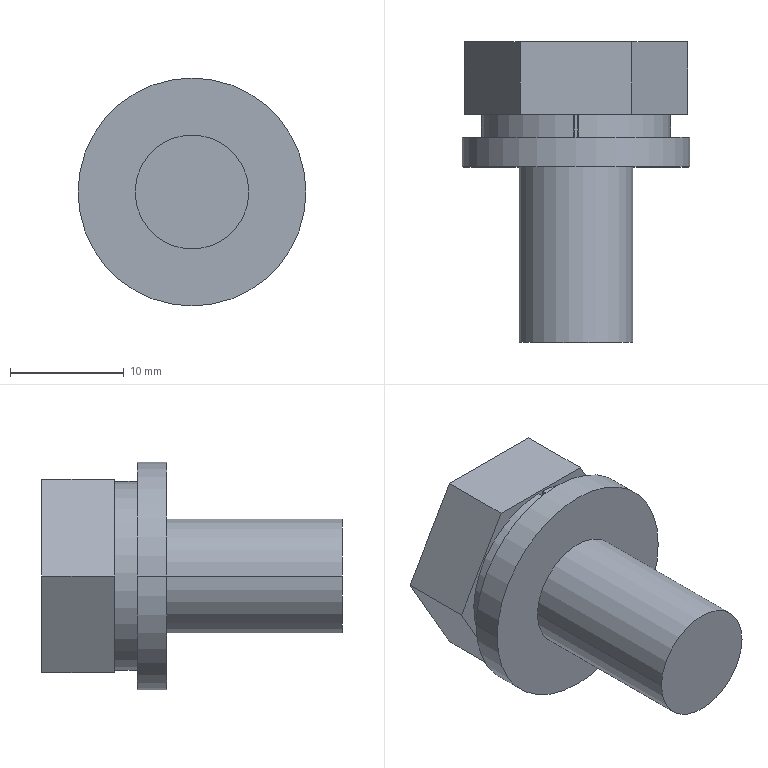Part | STEP file | LIB_68343151_M10X20 | 1 solid | 19 faces | box 20 x 26.4 x 20 mm | volume 4058 mm3 | plane 13 | cylinder 6 | commonest cylinder face diameters 10 x3 20 x2 16.6 x1
STEP:
#1=CARTESIAN_POINT('',(0.,0.,0.));
#2=DIRECTION('',(0.,0.,1.));
#3=DIRECTION('',(1.,0.,0.));
#4=AXIS2_PLACEMENT_3D('',#1,#2,#3);
#5=CARTESIAN_POINT('',(-4.907,0.,-8.5));
#6=VERTEX_POINT('',#5);
#7=CARTESIAN_POINT('',(-9.815,0.,0.));
#8=VERTEX_POINT('',#7);
#9=CARTESIAN_POINT('',(-4.907,0.,-8.5));
#10=DIRECTION('',(-0.5,0.,0.866));
#11=VECTOR('',#10,1.);
#12=LINE('',#9,#11);
#13=CARTESIAN_POINT('',(0.,0.,0.));
#14=DIRECTION('',(0.,1.,0.));
#15=DIRECTION('',(1.,0.,0.));
#16=AXIS2_PLACEMENT_3D('',#13,#14,#15);
#17=PLANE('',#16);
#18=CARTESIAN_POINT('',(-4.907,8.5));
#19=DIRECTION('',(-0.5,-0.866));
#20=VECTOR('',#19,1.);
#21=LINE('',#18,#20);
#22=(GEOMETRIC_REPRESENTATION_CONTEXT(2)PARAMETRIC_REPRESENTATION_CONTEXT()REPRESENTATION_CONTEXT('',''));
#23=DEFINITIONAL_REPRESENTATION('',(#21),#22);
#24=PCURVE('',#17,#23);
#25=CARTESIAN_POINT('',(-4.907,0.,-8.5));
#26=DIRECTION('',(-0.866,0.,-0.5));
#27=DIRECTION('',(-0.5,0.,0.866));
#28=AXIS2_PLACEMENT_3D('',#25,#26,#27);
#29=PLANE('',#28);
#30=CARTESIAN_POINT('',(0.,0.));
#31=DIRECTION('',(1.,0.));
#32=VECTOR('',#31,1.);
#33=LINE('',#30,#32);
#34=(GEOMETRIC_REPRESENTATION_CONTEXT(2)PARAMETRIC_REPRESENTATION_CONTEXT()REPRESENTATION_CONTEXT('',''));
#35=DEFINITIONAL_REPRESENTATION('',(#33),#34);
#36=PCURVE('',#29,#35);
#37=SURFACE_CURVE('',#12,(#24,#36),.PCURVE_S1.);
#38=EDGE_CURVE('',#6,#8,#37,.T.);
#39=ORIENTED_EDGE('',*,*,#38,.T.);
#40=CARTESIAN_POINT('',(-4.907,0.,8.5));
#41=VERTEX_POINT('',#40);
#42=CARTESIAN_POINT('',(-9.815,0.,0.));
#43=DIRECTION('',(0.5,0.,0.866));
#44=VECTOR('',#43,1.);
#45=LINE('',#42,#44);
#46=CARTESIAN_POINT('',(-9.815,0.));
#47=DIRECTION('',(0.5,-0.866));
#48=VECTOR('',#47,1.);
#49=LINE('',#46,#48);
#50=(GEOMETRIC_REPRESENTATION_CONTEXT(2)PARAMETRIC_REPRESENTATION_CONTEXT()REPRESENTATION_CONTEXT('',''));
#51=DEFINITIONAL_REPRESENTATION('',(#49),#50);
#52=PCURVE('',#17,#51);
#53=CARTESIAN_POINT('',(-9.815,0.,0.));
#54=DIRECTION('',(-0.866,0.,0.5));
#55=DIRECTION('',(0.5,0.,0.866));
#56=AXIS2_PLACEMENT_3D('',#53,#54,#55);
#57=PLANE('',#56);
#58=CARTESIAN_POINT('',(0.,0.));
#59=DIRECTION('',(1.,0.));
#60=VECTOR('',#59,1.);
#61=LINE('',#58,#60);
#62=(GEOMETRIC_REPRESENTATION_CONTEXT(2)PARAMETRIC_REPRESENTATION_CONTEXT()REPRESENTATION_CONTEXT('',''));
#63=DEFINITIONAL_REPRESENTATION('',(#61),#62);
#64=PCURVE('',#57,#63);
#65=SURFACE_CURVE('',#45,(#52,#64),.PCURVE_S1.);
#66=EDGE_CURVE('',#8,#41,#65,.T.);
#67=ORIENTED_EDGE('',*,*,#66,.T.);
#68=CARTESIAN_POINT('',(4.907,0.,8.5));
#69=VERTEX_POINT('',#68);
#70=CARTESIAN_POINT('',(-4.907,0.,8.5));
#71=DIRECTION('',(1.,0.,0.));
#72=VECTOR('',#71,1.);
#73=LINE('',#70,#72);
#74=CARTESIAN_POINT('',(-4.907,-8.5));
#75=DIRECTION('',(1.,0.));
#76=VECTOR('',#75,1.);
#77=LINE('',#74,#76);
#78=(GEOMETRIC_REPRESENTATION_CONTEXT(2)PARAMETRIC_REPRESENTATION_CONTEXT()REPRESENTATION_CONTEXT('',''));
#79=DEFINITIONAL_REPRESENTATION('',(#77),#78);
#80=PCURVE('',#17,#79);
#81=CARTESIAN_POINT('',(-4.907,0.,8.5));
#82=DIRECTION('',(0.,0.,1.));
#83=DIRECTION('',(1.,0.,0.));
#84=AXIS2_PLACEMENT_3D('',#81,#82,#83);
#85=PLANE('',#84);
#86=CARTESIAN_POINT('',(0.,0.));
#87=DIRECTION('',(1.,0.));
#88=VECTOR('',#87,1.);
#89=LINE('',#86,#88);
#90=(GEOMETRIC_REPRESENTATION_CONTEXT(2)PARAMETRIC_REPRESENTATION_CONTEXT()REPRESENTATION_CONTEXT('',''));
#91=DEFINITIONAL_REPRESENTATION('',(#89),#90);
#92=PCURVE('',#85,#91);
#93=SURFACE_CURVE('',#73,(#80,#92),.PCURVE_S1.);
#94=EDGE_CURVE('',#41,#69,#93,.T.);
#95=ORIENTED_EDGE('',*,*,#94,.T.);
#96=CARTESIAN_POINT('',(9.815,0.,0.));
#97=VERTEX_POINT('',#96);
#98=CARTESIAN_POINT('',(4.907,0.,8.5));
#99=DIRECTION('',(0.5,0.,-0.866));
#100=VECTOR('',#99,1.);
#101=LINE('',#98,#100);
#102=CARTESIAN_POINT('',(4.907,-8.5));
#103=DIRECTION('',(0.5,0.866));
#104=VECTOR('',#103,1.);
#105=LINE('',#102,#104);
#106=(GEOMETRIC_REPRESENTATION_CONTEXT(2)PARAMETRIC_REPRESENTATION_CONTEXT()REPRESENTATION_CONTEXT('',''));
#107=DEFINITIONAL_REPRESENTATION('',(#105),#106);
#108=PCURVE('',#17,#107);
#109=CARTESIAN_POINT('',(4.907,0.,8.5));
#110=DIRECTION('',(0.866,0.,0.5));
#111=DIRECTION('',(0.5,0.,-0.866));
#112=AXIS2_PLACEMENT_3D('',#109,#110,#111);
#113=PLANE('',#112);
#114=CARTESIAN_POINT('',(0.,0.));
#115=DIRECTION('',(1.,0.));
#116=VECTOR('',#115,1.);
#117=LINE('',#114,#116);
#118=(GEOMETRIC_REPRESENTATION_CONTEXT(2)PARAMETRIC_REPRESENTATION_CONTEXT()REPRESENTATION_CONTEXT('',''));
#119=DEFINITIONAL_REPRESENTATION('',(#117),#118);
#120=PCURVE('',#113,#119);
#121=SURFACE_CURVE('',#101,(#108,#120),.PCURVE_S1.);
#122=EDGE_CURVE('',#69,#97,#121,.T.);
#123=ORIENTED_EDGE('',*,*,#122,.T.);
#124=CARTESIAN_POINT('',(4.907,0.,-8.5));
#125=VERTEX_POINT('',#124);
#126=CARTESIAN_POINT('',(9.815,0.,0.));
#127=DIRECTION('',(-0.5,0.,-0.866));
#128=VECTOR('',#127,1.);
#129=LINE('',#126,#128);
#130=CARTESIAN_POINT('',(9.815,0.));
#131=DIRECTION('',(-0.5,0.866));
#132=VECTOR('',#131,1.);
#133=LINE('',#130,#132);
#134=(GEOMETRIC_REPRESENTATION_CONTEXT(2)PARAMETRIC_REPRESENTATION_CONTEXT()REPRESENTATION_CONTEXT('',''));
#135=DEFINITIONAL_REPRESENTATION('',(#133),#134);
#136=PCURVE('',#17,#135);
#137=CARTESIAN_POINT('',(9.815,0.,0.));
#138=DIRECTION('',(0.866,0.,-0.5));
#139=DIRECTION('',(-0.5,0.,-0.866));
#140=AXIS2_PLACEMENT_3D('',#137,#138,#139);
#141=PLANE('',#140);
#142=CARTESIAN_POINT('',(0.,0.));
#143=DIRECTION('',(1.,0.));
#144=VECTOR('',#143,1.);
#145=LINE('',#142,#144);
#146=(GEOMETRIC_REPRESENTATION_CONTEXT(2)PARAMETRIC_REPRESENTATION_CONTEXT()REPRESENTATION_CONTEXT('',''));
#147=DEFINITIONAL_REPRESENTATION('',(#145),#146);
#148=PCURVE('',#141,#147);
#149=SURFACE_CURVE('',#129,(#136,#148),.PCURVE_S1.);
#150=EDGE_CURVE('',#97,#125,#149,.T.);
#151=ORIENTED_EDGE('',*,*,#150,.T.);
#152=CARTESIAN_POINT('',(4.907,0.,-8.5));
#153=DIRECTION('',(-1.,0.,0.));
#154=VECTOR('',#153,1.);
#155=LINE('',#152,#154);
#156=CARTESIAN_POINT('',(4.907,8.5));
#157=DIRECTION('',(-1.,0.));
#158=VECTOR('',#157,1.);
#159=LINE('',#156,#158);
#160=(GEOMETRIC_REPRESENTATION_CONTEXT(2)PARAMETRIC_REPRESENTATION_CONTEXT()REPRESENTATION_CONTEXT('',''));
#161=DEFINITIONAL_REPRESENTATION('',(#159),#160);
#162=PCURVE('',#17,#161);
#163=CARTESIAN_POINT('',(4.907,0.,-8.5));
#164=DIRECTION('',(0.,0.,-1.));
#165=DIRECTION('',(-1.,0.,0.));
#166=AXIS2_PLACEMENT_3D('',#163,#164,#165);
#167=PLANE('',#166);
#168=CARTESIAN_POINT('',(0.,0.));
#169=DIRECTION('',(1.,0.));
#170=VECTOR('',#169,1.);
#171=LINE('',#168,#170);
#172=(GEOMETRIC_REPRESENTATION_CONTEXT(2)PARAMETRIC_REPRESENTATION_CONTEXT()REPRESENTATION_CONTEXT('',''));
#173=DEFINITIONAL_REPRESENTATION('',(#171),#172);
#174=PCURVE('',#167,#173);
#175=SURFACE_CURVE('',#155,(#162,#174),.PCURVE_S1.);
#176=EDGE_CURVE('',#125,#6,#175,.T.);
#177=ORIENTED_EDGE('',*,*,#176,.T.);
#178=EDGE_LOOP('',(#39,#67,#95,#123,#151,#177));
#179=FACE_BOUND('',#178,.F.);
#180=CARTESIAN_POINT('',(-0.25,0.,8.296));
#181=VERTEX_POINT('',#180);
#182=CARTESIAN_POINT('',(0.25,0.,8.296));
#183=VERTEX_POINT('',#182);
#184=CARTESIAN_POINT('',(0.,0.,0.));
#185=DIRECTION('',(0.,-1.,0.));
#186=DIRECTION('',(-0.03012,0.,0.9995));
#187=AXIS2_PLACEMENT_3D('',#184,#185,#186);
#188=CIRCLE('',#187,8.3);
#189=CARTESIAN_POINT('',(-0.25,-8.296));
#190=CARTESIAN_POINT('',(-14.619,-7.863));
#191=CARTESIAN_POINT('',(-7.06,4.365));
#192=CARTESIAN_POINT('',(0.5,16.592));
#193=CARTESIAN_POINT('',(7.31,3.932));
#194=CARTESIAN_POINT('',(14.119,-8.729));
#195=CARTESIAN_POINT('',(-0.25,-8.296));
#196=(BOUNDED_CURVE()B_SPLINE_CURVE(2,(#189,#190,#191,#192,#193,#194,#195),.UNSPECIFIED.,.T.,.F.)B_SPLINE_CURVE_WITH_KNOTS((1,2,2,2,2,1),(-2.094,0.,2.094,4.189,6.283,8.378),.UNSPECIFIED.)CURVE()GEOMETRIC_REPRESENTATION_ITEM()RATIONAL_B_SPLINE_CURVE((1.,0.5,1.,0.5,1.,0.5,1.))REPRESENTATION_ITEM(''));
#197=(GEOMETRIC_REPRESENTATION_CONTEXT(2)PARAMETRIC_REPRESENTATION_CONTEXT()REPRESENTATION_CONTEXT('',''));
#198=DEFINITIONAL_REPRESENTATION('',(#196),#197);
#199=PCURVE('',#17,#198);
#200=CARTESIAN_POINT('',(0.,0.,0.));
#201=DIRECTION('',(0.,-1.,0.));
#202=DIRECTION('',(0.,0.,-1.));
#203=AXIS2_PLACEMENT_3D('',#200,#201,#202);
#204=CYLINDRICAL_SURFACE('',#203,8.3);
#205=CARTESIAN_POINT('',(3.172,0.));
#206=DIRECTION('',(1.,0.));
#207=VECTOR('',#206,1.);
#208=LINE('',#205,#207);
#209=(GEOMETRIC_REPRESENTATION_CONTEXT(2)PARAMETRIC_REPRESENTATION_CONTEXT()REPRESENTATION_CONTEXT('',''));
#210=DEFINITIONAL_REPRESENTATION('',(#208),#209);
#211=PCURVE('',#204,#210);
#212=SURFACE_CURVE('',#188,(#199,#211),.PCURVE_S1.);
#213=EDGE_CURVE('',#181,#183,#212,.T.);
#214=ORIENTED_EDGE('',*,*,#213,.T.);
#215=CARTESIAN_POINT('',(0.1506,0.,4.998));
#216=VERTEX_POINT('',#215);
#217=CARTESIAN_POINT('',(0.25,0.,8.296));
#218=DIRECTION('',(-0.03012,0.,-0.9995));
#219=VECTOR('',#218,1.);
#220=LINE('',#217,#219);
#221=CARTESIAN_POINT('',(0.25,-8.296));
#222=DIRECTION('',(-0.03012,0.9995));
#223=VECTOR('',#222,1.);
#224=LINE('',#221,#223);
#225=(GEOMETRIC_REPRESENTATION_CONTEXT(2)PARAMETRIC_REPRESENTATION_CONTEXT()REPRESENTATION_CONTEXT('',''));
#226=DEFINITIONAL_REPRESENTATION('',(#224),#225);
#227=PCURVE('',#17,#226);
#228=CARTESIAN_POINT('',(0.25,0.,8.296));
#229=DIRECTION('',(-0.9995,0.,0.03012));
#230=DIRECTION('',(-0.03012,0.,-0.9995));
#231=AXIS2_PLACEMENT_3D('',#228,#229,#230);
#232=PLANE('',#231);
#233=CARTESIAN_POINT('',(0.,0.));
#234=DIRECTION('',(1.,0.));
#235=VECTOR('',#234,1.);
#236=LINE('',#233,#235);
#237=(GEOMETRIC_REPRESENTATION_CONTEXT(2)PARAMETRIC_REPRESENTATION_CONTEXT()REPRESENTATION_CONTEXT('',''));
#238=DEFINITIONAL_REPRESENTATION('',(#236),#237);
#239=PCURVE('',#232,#238);
#240=SURFACE_CURVE('',#220,(#227,#239),.PCURVE_S1.);
#241=EDGE_CURVE('',#183,#216,#240,.T.);
#242=ORIENTED_EDGE('',*,*,#241,.T.);
#243=CARTESIAN_POINT('',(-0.1506,0.,4.998));
#244=VERTEX_POINT('',#243);
#245=CARTESIAN_POINT('',(0.,0.,0.));
#246=DIRECTION('',(0.,-1.,0.));
#247=DIRECTION('',(0.03012,0.,0.9995));
#248=AXIS2_PLACEMENT_3D('',#245,#246,#247);
#249=CIRCLE('',#248,5.);
#250=CARTESIAN_POINT('',(0.1506,-4.998));
#251=CARTESIAN_POINT('',(-8.506,-5.259));
#252=CARTESIAN_POINT('',(-4.403,2.368));
#253=CARTESIAN_POINT('',(-0.3012,9.995));
#254=CARTESIAN_POINT('',(4.253,2.629));
#255=CARTESIAN_POINT('',(8.807,-4.737));
#256=CARTESIAN_POINT('',(0.1506,-4.998));
#257=(BOUNDED_CURVE()B_SPLINE_CURVE(2,(#250,#251,#252,#253,#254,#255,#256),.UNSPECIFIED.,.T.,.F.)B_SPLINE_CURVE_WITH_KNOTS((1,2,2,2,2,1),(-2.094,0.,2.094,4.189,6.283,8.378),.UNSPECIFIED.)CURVE()GEOMETRIC_REPRESENTATION_ITEM()RATIONAL_B_SPLINE_CURVE((1.,0.5,1.,0.5,1.,0.5,1.))REPRESENTATION_ITEM(''));
#258=(GEOMETRIC_REPRESENTATION_CONTEXT(2)PARAMETRIC_REPRESENTATION_CONTEXT()REPRESENTATION_CONTEXT('',''));
#259=DEFINITIONAL_REPRESENTATION('',(#257),#258);
#260=PCURVE('',#17,#259);
#261=CARTESIAN_POINT('',(0.,0.,0.));
#262=DIRECTION('',(0.,-1.,0.));
#263=DIRECTION('',(1.,0.,0.));
#264=AXIS2_PLACEMENT_3D('',#261,#262,#263);
#265=CYLINDRICAL_SURFACE('',#264,5.);
#266=CARTESIAN_POINT('',(1.541,0.));
#267=DIRECTION('',(1.,0.));
#268=VECTOR('',#267,1.);
#269=LINE('',#266,#268);
#270=(GEOMETRIC_REPRESENTATION_CONTEXT(2)PARAMETRIC_REPRESENTATION_CONTEXT()REPRESENTATION_CONTEXT('',''));
#271=DEFINITIONAL_REPRESENTATION('',(#269),#270);
#272=PCURVE('',#265,#271);
#273=SURFACE_CURVE('',#249,(#260,#272),.PCURVE_S1.);
#274=EDGE_CURVE('',#216,#244,#273,.T.);
#275=ORIENTED_EDGE('',*,*,#274,.T.);
#276=CARTESIAN_POINT('',(-0.1506,0.,4.998));
#277=DIRECTION('',(-0.03012,0.,0.9995));
#278=VECTOR('',#277,1.);
#279=LINE('',#276,#278);
#280=CARTESIAN_POINT('',(-0.1506,-4.998));
#281=DIRECTION('',(-0.03012,-0.9995));
#282=VECTOR('',#281,1.);
#283=LINE('',#280,#282);
#284=(GEOMETRIC_REPRESENTATION_CONTEXT(2)PARAMETRIC_REPRESENTATION_CONTEXT()REPRESENTATION_CONTEXT('',''));
#285=DEFINITIONAL_REPRESENTATION('',(#283),#284);
#286=PCURVE('',#17,#285);
#287=CARTESIAN_POINT('',(-0.1506,0.,4.998));
#288=DIRECTION('',(0.9995,0.,0.03012));
#289=DIRECTION('',(-0.03012,0.,0.9995));
#290=AXIS2_PLACEMENT_3D('',#287,#288,#289);
#291=PLANE('',#290);
#292=CARTESIAN_POINT('',(0.,0.));
#293=DIRECTION('',(1.,0.));
#294=VECTOR('',#293,1.);
#295=LINE('',#292,#294);
#296=(GEOMETRIC_REPRESENTATION_CONTEXT(2)PARAMETRIC_REPRESENTATION_CONTEXT()REPRESENTATION_CONTEXT('',''));
#297=DEFINITIONAL_REPRESENTATION('',(#295),#296);
#298=PCURVE('',#291,#297);
#299=SURFACE_CURVE('',#279,(#286,#298),.PCURVE_S1.);
#300=EDGE_CURVE('',#244,#181,#299,.T.);
#301=ORIENTED_EDGE('',*,*,#300,.T.);
#302=EDGE_LOOP('',(#214,#242,#275,#301));
#303=FACE_BOUND('',#302,.F.);
#304=ADVANCED_FACE('',(#179,#303),#17,.F.);
#305=ORIENTED_EDGE('',*,*,#38,.F.);
#306=CARTESIAN_POINT('',(-4.907,6.4,-8.5));
#307=VERTEX_POINT('',#306);
#308=CARTESIAN_POINT('',(-4.907,0.,-8.5));
#309=DIRECTION('',(0.,1.,0.));
#310=VECTOR('',#309,1.);
#311=LINE('',#308,#310);
#312=CARTESIAN_POINT('',(0.,0.));
#313=DIRECTION('',(0.,1.));
#314=VECTOR('',#313,1.);
#315=LINE('',#312,#314);
#316=(GEOMETRIC_REPRESENTATION_CONTEXT(2)PARAMETRIC_REPRESENTATION_CONTEXT()REPRESENTATION_CONTEXT('',''));
#317=DEFINITIONAL_REPRESENTATION('',(#315),#316);
#318=PCURVE('',#29,#317);
#319=CARTESIAN_POINT('',(9.815,0.));
#320=DIRECTION('',(0.,1.));
#321=VECTOR('',#320,1.);
#322=LINE('',#319,#321);
#323=(GEOMETRIC_REPRESENTATION_CONTEXT(2)PARAMETRIC_REPRESENTATION_CONTEXT()REPRESENTATION_CONTEXT('',''));
#324=DEFINITIONAL_REPRESENTATION('',(#322),#323);
#325=PCURVE('',#167,#324);
#326=SURFACE_CURVE('',#311,(#318,#325),.PCURVE_S1.);
#327=EDGE_CURVE('',#6,#307,#326,.T.);
#328=ORIENTED_EDGE('',*,*,#327,.T.);
#329=CARTESIAN_POINT('',(-9.815,6.4,0.));
#330=VERTEX_POINT('',#329);
#331=CARTESIAN_POINT('',(-4.907,6.4,-8.5));
#332=DIRECTION('',(-0.5,0.,0.866));
#333=VECTOR('',#332,1.);
#334=LINE('',#331,#333);
#335=CARTESIAN_POINT('',(0.,6.4));
#336=DIRECTION('',(1.,0.));
#337=VECTOR('',#336,1.);
#338=LINE('',#335,#337);
#339=(GEOMETRIC_REPRESENTATION_CONTEXT(2)PARAMETRIC_REPRESENTATION_CONTEXT()REPRESENTATION_CONTEXT('',''));
#340=DEFINITIONAL_REPRESENTATION('',(#338),#339);
#341=PCURVE('',#29,#340);
#342=CARTESIAN_POINT('',(0.,6.4,0.));
#343=DIRECTION('',(0.,1.,0.));
#344=DIRECTION('',(1.,0.,0.));
#345=AXIS2_PLACEMENT_3D('',#342,#343,#344);
#346=PLANE('',#345);
#347=CARTESIAN_POINT('',(-4.907,8.5));
#348=DIRECTION('',(-0.5,-0.866));
#349=VECTOR('',#348,1.);
#350=LINE('',#347,#349);
#351=(GEOMETRIC_REPRESENTATION_CONTEXT(2)PARAMETRIC_REPRESENTATION_CONTEXT()REPRESENTATION_CONTEXT('',''));
#352=DEFINITIONAL_REPRESENTATION('',(#350),#351);
#353=PCURVE('',#346,#352);
#354=SURFACE_CURVE('',#334,(#341,#353),.PCURVE_S1.);
#355=EDGE_CURVE('',#307,#330,#354,.T.);
#356=ORIENTED_EDGE('',*,*,#355,.T.);
#357=CARTESIAN_POINT('',(-9.815,0.,0.));
#358=DIRECTION('',(0.,1.,0.));
#359=VECTOR('',#358,1.);
#360=LINE('',#357,#359);
#361=CARTESIAN_POINT('',(9.815,0.));
#362=DIRECTION('',(0.,1.));
#363=VECTOR('',#362,1.);
#364=LINE('',#361,#363);
#365=(GEOMETRIC_REPRESENTATION_CONTEXT(2)PARAMETRIC_REPRESENTATION_CONTEXT()REPRESENTATION_CONTEXT('',''));
#366=DEFINITIONAL_REPRESENTATION('',(#364),#365);
#367=PCURVE('',#29,#366);
#368=CARTESIAN_POINT('',(0.,0.));
#369=DIRECTION('',(0.,1.));
#370=VECTOR('',#369,1.);
#371=LINE('',#368,#370);
#372=(GEOMETRIC_REPRESENTATION_CONTEXT(2)PARAMETRIC_REPRESENTATION_CONTEXT()REPRESENTATION_CONTEXT('',''));
#373=DEFINITIONAL_REPRESENTATION('',(#371),#372);
#374=PCURVE('',#57,#373);
#375=SURFACE_CURVE('',#360,(#367,#374),.PCURVE_S1.);
#376=EDGE_CURVE('',#8,#330,#375,.T.);
#377=ORIENTED_EDGE('',*,*,#376,.F.);
#378=EDGE_LOOP('',(#305,#328,#356,#377));
#379=FACE_BOUND('',#378,.F.);
#380=ADVANCED_FACE('',(#379),#29,.T.);
#381=ORIENTED_EDGE('',*,*,#176,.F.);
#382=CARTESIAN_POINT('',(4.907,6.4,-8.5));
#383=VERTEX_POINT('',#382);
#384=CARTESIAN_POINT('',(4.907,0.,-8.5));
#385=DIRECTION('',(0.,1.,0.));
#386=VECTOR('',#385,1.);
#387=LINE('',#384,#386);
#388=CARTESIAN_POINT('',(0.,0.));
#389=DIRECTION('',(0.,1.));
#390=VECTOR('',#389,1.);
#391=LINE('',#388,#390);
#392=(GEOMETRIC_REPRESENTATION_CONTEXT(2)PARAMETRIC_REPRESENTATION_CONTEXT()REPRESENTATION_CONTEXT('',''));
#393=DEFINITIONAL_REPRESENTATION('',(#391),#392);
#394=PCURVE('',#167,#393);
#395=CARTESIAN_POINT('',(9.815,0.));
#396=DIRECTION('',(0.,1.));
#397=VECTOR('',#396,1.);
#398=LINE('',#395,#397);
#399=(GEOMETRIC_REPRESENTATION_CONTEXT(2)PARAMETRIC_REPRESENTATION_CONTEXT()REPRESENTATION_CONTEXT('',''));
#400=DEFINITIONAL_REPRESENTATION('',(#398),#399);
#401=PCURVE('',#141,#400);
#402=SURFACE_CURVE('',#387,(#394,#401),.PCURVE_S1.);
#403=EDGE_CURVE('',#125,#383,#402,.T.);
#404=ORIENTED_EDGE('',*,*,#403,.T.);
#405=CARTESIAN_POINT('',(4.907,6.4,-8.5));
#406=DIRECTION('',(-1.,0.,0.));
#407=VECTOR('',#406,1.);
#408=LINE('',#405,#407);
#409=CARTESIAN_POINT('',(0.,6.4));
#410=DIRECTION('',(1.,0.));
#411=VECTOR('',#410,1.);
#412=LINE('',#409,#411);
#413=(GEOMETRIC_REPRESENTATION_CONTEXT(2)PARAMETRIC_REPRESENTATION_CONTEXT()REPRESENTATION_CONTEXT('',''));
#414=DEFINITIONAL_REPRESENTATION('',(#412),#413);
#415=PCURVE('',#167,#414);
#416=CARTESIAN_POINT('',(4.907,8.5));
#417=DIRECTION('',(-1.,0.));
#418=VECTOR('',#417,1.);
#419=LINE('',#416,#418);
#420=(GEOMETRIC_REPRESENTATION_CONTEXT(2)PARAMETRIC_REPRESENTATION_CONTEXT()REPRESENTATION_CONTEXT('',''));
#421=DEFINITIONAL_REPRESENTATION('',(#419),#420);
#422=PCURVE('',#346,#421);
#423=SURFACE_CURVE('',#408,(#415,#422),.PCURVE_S1.);
#424=EDGE_CURVE('',#383,#307,#423,.T.);
#425=ORIENTED_EDGE('',*,*,#424,.T.);
#426=ORIENTED_EDGE('',*,*,#327,.F.);
#427=EDGE_LOOP('',(#381,#404,#425,#426));
#428=FACE_BOUND('',#427,.F.);
#429=ADVANCED_FACE('',(#428),#167,.T.);
#430=ORIENTED_EDGE('',*,*,#150,.F.);
#431=CARTESIAN_POINT('',(9.815,6.4,0.));
#432=VERTEX_POINT('',#431);
#433=CARTESIAN_POINT('',(9.815,0.,0.));
#434=DIRECTION('',(0.,1.,0.));
#435=VECTOR('',#434,1.);
#436=LINE('',#433,#435);
#437=CARTESIAN_POINT('',(0.,0.));
#438=DIRECTION('',(0.,1.));
#439=VECTOR('',#438,1.);
#440=LINE('',#437,#439);
#441=(GEOMETRIC_REPRESENTATION_CONTEXT(2)PARAMETRIC_REPRESENTATION_CONTEXT()REPRESENTATION_CONTEXT('',''));
#442=DEFINITIONAL_REPRESENTATION('',(#440),#441);
#443=PCURVE('',#141,#442);
#444=CARTESIAN_POINT('',(9.815,0.));
#445=DIRECTION('',(0.,1.));
#446=VECTOR('',#445,1.);
#447=LINE('',#444,#446);
#448=(GEOMETRIC_REPRESENTATION_CONTEXT(2)PARAMETRIC_REPRESENTATION_CONTEXT()REPRESENTATION_CONTEXT('',''));
#449=DEFINITIONAL_REPRESENTATION('',(#447),#448);
#450=PCURVE('',#113,#449);
#451=SURFACE_CURVE('',#436,(#443,#450),.PCURVE_S1.);
#452=EDGE_CURVE('',#97,#432,#451,.T.);
#453=ORIENTED_EDGE('',*,*,#452,.T.);
#454=CARTESIAN_POINT('',(9.815,6.4,0.));
#455=DIRECTION('',(-0.5,0.,-0.866));
#456=VECTOR('',#455,1.);
#457=LINE('',#454,#456);
#458=CARTESIAN_POINT('',(0.,6.4));
#459=DIRECTION('',(1.,0.));
#460=VECTOR('',#459,1.);
#461=LINE('',#458,#460);
#462=(GEOMETRIC_REPRESENTATION_CONTEXT(2)PARAMETRIC_REPRESENTATION_CONTEXT()REPRESENTATION_CONTEXT('',''));
#463=DEFINITIONAL_REPRESENTATION('',(#461),#462);
#464=PCURVE('',#141,#463);
#465=CARTESIAN_POINT('',(9.815,0.));
#466=DIRECTION('',(-0.5,0.866));
#467=VECTOR('',#466,1.);
#468=LINE('',#465,#467);
#469=(GEOMETRIC_REPRESENTATION_CONTEXT(2)PARAMETRIC_REPRESENTATION_CONTEXT()REPRESENTATION_CONTEXT('',''));
#470=DEFINITIONAL_REPRESENTATION('',(#468),#469);
#471=PCURVE('',#346,#470);
#472=SURFACE_CURVE('',#457,(#464,#471),.PCURVE_S1.);
#473=EDGE_CURVE('',#432,#383,#472,.T.);
#474=ORIENTED_EDGE('',*,*,#473,.T.);
#475=ORIENTED_EDGE('',*,*,#403,.F.);
#476=EDGE_LOOP('',(#430,#453,#474,#475));
#477=FACE_BOUND('',#476,.F.);
#478=ADVANCED_FACE('',(#477),#141,.T.);
#479=ORIENTED_EDGE('',*,*,#122,.F.);
#480=CARTESIAN_POINT('',(4.907,6.4,8.5));
#481=VERTEX_POINT('',#480);
#482=CARTESIAN_POINT('',(4.907,0.,8.5));
#483=DIRECTION('',(0.,1.,0.));
#484=VECTOR('',#483,1.);
#485=LINE('',#482,#484);
#486=CARTESIAN_POINT('',(0.,0.));
#487=DIRECTION('',(0.,1.));
#488=VECTOR('',#487,1.);
#489=LINE('',#486,#488);
#490=(GEOMETRIC_REPRESENTATION_CONTEXT(2)PARAMETRIC_REPRESENTATION_CONTEXT()REPRESENTATION_CONTEXT('',''));
#491=DEFINITIONAL_REPRESENTATION('',(#489),#490);
#492=PCURVE('',#113,#491);
#493=CARTESIAN_POINT('',(9.815,0.));
#494=DIRECTION('',(0.,1.));
#495=VECTOR('',#494,1.);
#496=LINE('',#493,#495);
#497=(GEOMETRIC_REPRESENTATION_CONTEXT(2)PARAMETRIC_REPRESENTATION_CONTEXT()REPRESENTATION_CONTEXT('',''));
#498=DEFINITIONAL_REPRESENTATION('',(#496),#497);
#499=PCURVE('',#85,#498);
#500=SURFACE_CURVE('',#485,(#492,#499),.PCURVE_S1.);
#501=EDGE_CURVE('',#69,#481,#500,.T.);
#502=ORIENTED_EDGE('',*,*,#501,.T.);
#503=CARTESIAN_POINT('',(4.907,6.4,8.5));
#504=DIRECTION('',(0.5,0.,-0.866));
#505=VECTOR('',#504,1.);
#506=LINE('',#503,#505);
#507=CARTESIAN_POINT('',(0.,6.4));
#508=DIRECTION('',(1.,0.));
#509=VECTOR('',#508,1.);
#510=LINE('',#507,#509);
#511=(GEOMETRIC_REPRESENTATION_CONTEXT(2)PARAMETRIC_REPRESENTATION_CONTEXT()REPRESENTATION_CONTEXT('',''));
#512=DEFINITIONAL_REPRESENTATION('',(#510),#511);
#513=PCURVE('',#113,#512);
#514=CARTESIAN_POINT('',(4.907,-8.5));
#515=DIRECTION('',(0.5,0.866));
#516=VECTOR('',#515,1.);
#517=LINE('',#514,#516);
#518=(GEOMETRIC_REPRESENTATION_CONTEXT(2)PARAMETRIC_REPRESENTATION_CONTEXT()REPRESENTATION_CONTEXT('',''));
#519=DEFINITIONAL_REPRESENTATION('',(#517),#518);
#520=PCURVE('',#346,#519);
#521=SURFACE_CURVE('',#506,(#513,#520),.PCURVE_S1.);
#522=EDGE_CURVE('',#481,#432,#521,.T.);
#523=ORIENTED_EDGE('',*,*,#522,.T.);
#524=ORIENTED_EDGE('',*,*,#452,.F.);
#525=EDGE_LOOP('',(#479,#502,#523,#524));
#526=FACE_BOUND('',#525,.F.);
#527=ADVANCED_FACE('',(#526),#113,.T.);
#528=ORIENTED_EDGE('',*,*,#94,.F.);
#529=CARTESIAN_POINT('',(-4.907,6.4,8.5));
#530=VERTEX_POINT('',#529);
#531=CARTESIAN_POINT('',(-4.907,0.,8.5));
#532=DIRECTION('',(0.,1.,0.));
#533=VECTOR('',#532,1.);
#534=LINE('',#531,#533);
#535=CARTESIAN_POINT('',(0.,0.));
#536=DIRECTION('',(0.,1.));
#537=VECTOR('',#536,1.);
#538=LINE('',#535,#537);
#539=(GEOMETRIC_REPRESENTATION_CONTEXT(2)PARAMETRIC_REPRESENTATION_CONTEXT()REPRESENTATION_CONTEXT('',''));
#540=DEFINITIONAL_REPRESENTATION('',(#538),#539);
#541=PCURVE('',#85,#540);
#542=CARTESIAN_POINT('',(9.815,0.));
#543=DIRECTION('',(0.,1.));
#544=VECTOR('',#543,1.);
#545=LINE('',#542,#544);
#546=(GEOMETRIC_REPRESENTATION_CONTEXT(2)PARAMETRIC_REPRESENTATION_CONTEXT()REPRESENTATION_CONTEXT('',''));
#547=DEFINITIONAL_REPRESENTATION('',(#545),#546);
#548=PCURVE('',#57,#547);
#549=SURFACE_CURVE('',#534,(#541,#548),.PCURVE_S1.);
#550=EDGE_CURVE('',#41,#530,#549,.T.);
#551=ORIENTED_EDGE('',*,*,#550,.T.);
#552=CARTESIAN_POINT('',(-4.907,6.4,8.5));
#553=DIRECTION('',(1.,0.,0.));
#554=VECTOR('',#553,1.);
#555=LINE('',#552,#554);
#556=CARTESIAN_POINT('',(0.,6.4));
#557=DIRECTION('',(1.,0.));
#558=VECTOR('',#557,1.);
#559=LINE('',#556,#558);
#560=(GEOMETRIC_REPRESENTATION_CONTEXT(2)PARAMETRIC_REPRESENTATION_CONTEXT()REPRESENTATION_CONTEXT('',''));
#561=DEFINITIONAL_REPRESENTATION('',(#559),#560);
#562=PCURVE('',#85,#561);
#563=CARTESIAN_POINT('',(-4.907,-8.5));
#564=DIRECTION('',(1.,0.));
#565=VECTOR('',#564,1.);
#566=LINE('',#563,#565);
#567=(GEOMETRIC_REPRESENTATION_CONTEXT(2)PARAMETRIC_REPRESENTATION_CONTEXT()REPRESENTATION_CONTEXT('',''));
#568=DEFINITIONAL_REPRESENTATION('',(#566),#567);
#569=PCURVE('',#346,#568);
#570=SURFACE_CURVE('',#555,(#562,#569),.PCURVE_S1.);
#571=EDGE_CURVE('',#530,#481,#570,.T.);
#572=ORIENTED_EDGE('',*,*,#571,.T.);
#573=ORIENTED_EDGE('',*,*,#501,.F.);
#574=EDGE_LOOP('',(#528,#551,#572,#573));
#575=FACE_BOUND('',#574,.F.);
#576=ADVANCED_FACE('',(#575),#85,.T.);
#577=ORIENTED_EDGE('',*,*,#66,.F.);
#578=ORIENTED_EDGE('',*,*,#376,.T.);
#579=CARTESIAN_POINT('',(-9.815,6.4,0.));
#580=DIRECTION('',(0.5,0.,0.866));
#581=VECTOR('',#580,1.);
#582=LINE('',#579,#581);
#583=CARTESIAN_POINT('',(0.,6.4));
#584=DIRECTION('',(1.,0.));
#585=VECTOR('',#584,1.);
#586=LINE('',#583,#585);
#587=(GEOMETRIC_REPRESENTATION_CONTEXT(2)PARAMETRIC_REPRESENTATION_CONTEXT()REPRESENTATION_CONTEXT('',''));
#588=DEFINITIONAL_REPRESENTATION('',(#586),#587);
#589=PCURVE('',#57,#588);
#590=CARTESIAN_POINT('',(-9.815,0.));
#591=DIRECTION('',(0.5,-0.866));
#592=VECTOR('',#591,1.);
#593=LINE('',#590,#592);
#594=(GEOMETRIC_REPRESENTATION_CONTEXT(2)PARAMETRIC_REPRESENTATION_CONTEXT()REPRESENTATION_CONTEXT('',''));
#595=DEFINITIONAL_REPRESENTATION('',(#593),#594);
#596=PCURVE('',#346,#595);
#597=SURFACE_CURVE('',#582,(#589,#596),.PCURVE_S1.);
#598=EDGE_CURVE('',#330,#530,#597,.T.);
#599=ORIENTED_EDGE('',*,*,#598,.T.);
#600=ORIENTED_EDGE('',*,*,#550,.F.);
#601=EDGE_LOOP('',(#577,#578,#599,#600));
#602=FACE_BOUND('',#601,.F.);
#603=ADVANCED_FACE('',(#602),#57,.T.);
#604=ORIENTED_EDGE('',*,*,#355,.F.);
#605=ORIENTED_EDGE('',*,*,#424,.F.);
#606=ORIENTED_EDGE('',*,*,#473,.F.);
#607=ORIENTED_EDGE('',*,*,#522,.F.);
#608=ORIENTED_EDGE('',*,*,#571,.F.);
#609=ORIENTED_EDGE('',*,*,#598,.F.);
#610=EDGE_LOOP('',(#604,#605,#606,#607,#608,#609));
#611=FACE_BOUND('',#610,.F.);
#612=ADVANCED_FACE('',(#611),#346,.T.);
#613=CARTESIAN_POINT('',(-0.25,-2.,8.296));
#614=VERTEX_POINT('',#613);
#615=CARTESIAN_POINT('',(-0.25,0.,8.296));
#616=DIRECTION('',(0.,-1.,0.));
#617=VECTOR('',#616,1.);
#618=LINE('',#615,#617);
#619=CARTESIAN_POINT('',(3.172,0.));
#620=DIRECTION('',(0.,1.));
#621=VECTOR('',#620,1.);
#622=LINE('',#619,#621);
#623=(GEOMETRIC_REPRESENTATION_CONTEXT(2)PARAMETRIC_REPRESENTATION_CONTEXT()REPRESENTATION_CONTEXT('',''));
#624=DEFINITIONAL_REPRESENTATION('',(#622),#623);
#625=PCURVE('',#204,#624);
#626=CARTESIAN_POINT('',(3.3,0.));
#627=DIRECTION('',(0.,1.));
#628=VECTOR('',#627,1.);
#629=LINE('',#626,#628);
#630=(GEOMETRIC_REPRESENTATION_CONTEXT(2)PARAMETRIC_REPRESENTATION_CONTEXT()REPRESENTATION_CONTEXT('',''));
#631=DEFINITIONAL_REPRESENTATION('',(#629),#630);
#632=PCURVE('',#291,#631);
#633=SURFACE_CURVE('',#618,(#625,#632),.PCURVE_S1.);
#634=EDGE_CURVE('',#181,#614,#633,.T.);
#635=ORIENTED_EDGE('',*,*,#634,.F.);
#636=ORIENTED_EDGE('',*,*,#213,.T.);
#637=CARTESIAN_POINT('',(0.25,-2.,8.296));
#638=VERTEX_POINT('',#637);
#639=CARTESIAN_POINT('',(0.25,0.,8.296));
#640=DIRECTION('',(0.,-1.,0.));
#641=VECTOR('',#640,1.);
#642=LINE('',#639,#641);
#643=CARTESIAN_POINT('',(9.395,0.));
#644=DIRECTION('',(0.,1.));
#645=VECTOR('',#644,1.);
#646=LINE('',#643,#645);
#647=(GEOMETRIC_REPRESENTATION_CONTEXT(2)PARAMETRIC_REPRESENTATION_CONTEXT()REPRESENTATION_CONTEXT('',''));
#648=DEFINITIONAL_REPRESENTATION('',(#646),#647);
#649=PCURVE('',#204,#648);
#650=CARTESIAN_POINT('',(0.,0.));
#651=DIRECTION('',(0.,1.));
#652=VECTOR('',#651,1.);
#653=LINE('',#650,#652);
#654=(GEOMETRIC_REPRESENTATION_CONTEXT(2)PARAMETRIC_REPRESENTATION_CONTEXT()REPRESENTATION_CONTEXT('',''));
#655=DEFINITIONAL_REPRESENTATION('',(#653),#654);
#656=PCURVE('',#232,#655);
#657=SURFACE_CURVE('',#642,(#649,#656),.PCURVE_S1.);
#658=EDGE_CURVE('',#183,#638,#657,.T.);
#659=ORIENTED_EDGE('',*,*,#658,.T.);
#660=CARTESIAN_POINT('',(0.,-2.,0.));
#661=DIRECTION('',(0.,-1.,0.));
#662=DIRECTION('',(-0.03012,0.,0.9995));
#663=AXIS2_PLACEMENT_3D('',#660,#661,#662);
#664=CIRCLE('',#663,8.3);
#665=CARTESIAN_POINT('',(3.172,2.));
#666=DIRECTION('',(1.,0.));
#667=VECTOR('',#666,1.);
#668=LINE('',#665,#667);
#669=(GEOMETRIC_REPRESENTATION_CONTEXT(2)PARAMETRIC_REPRESENTATION_CONTEXT()REPRESENTATION_CONTEXT('',''));
#670=DEFINITIONAL_REPRESENTATION('',(#668),#669);
#671=PCURVE('',#204,#670);
#672=CARTESIAN_POINT('',(0.,-2.,0.));
#673=DIRECTION('',(0.,-1.,0.));
#674=DIRECTION('',(1.,0.,0.));
#675=AXIS2_PLACEMENT_3D('',#672,#673,#674);
#676=PLANE('',#675);
#677=CARTESIAN_POINT('',(0.,0.));
#678=DIRECTION('',(-0.03012,0.9995));
#679=AXIS2_PLACEMENT_2D('',#677,#678);
#680=CIRCLE('',#679,8.3);
#681=(GEOMETRIC_REPRESENTATION_CONTEXT(2)PARAMETRIC_REPRESENTATION_CONTEXT()REPRESENTATION_CONTEXT('',''));
#682=DEFINITIONAL_REPRESENTATION('',(#680),#681);
#683=PCURVE('',#676,#682);
#684=SURFACE_CURVE('',#664,(#671,#683),.PCURVE_S1.);
#685=EDGE_CURVE('',#614,#638,#684,.T.);
#686=ORIENTED_EDGE('',*,*,#685,.F.);
#687=EDGE_LOOP('',(#635,#636,#659,#686));
#688=FACE_BOUND('',#687,.T.);
#689=ADVANCED_FACE('',(#688),#204,.T.);
#690=CARTESIAN_POINT('',(10.,-2.,0.));
#691=VERTEX_POINT('',#690);
#692=CARTESIAN_POINT('',(-10.,-2.,0.));
#693=VERTEX_POINT('',#692);
#694=CARTESIAN_POINT('',(0.,-2.,0.));
#695=DIRECTION('',(0.,-1.,0.));
#696=DIRECTION('',(1.,0.,0.));
#697=AXIS2_PLACEMENT_3D('',#694,#695,#696);
#698=CIRCLE('',#697,10.);
#699=CARTESIAN_POINT('',(0.,0.));
#700=DIRECTION('',(1.,0.));
#701=AXIS2_PLACEMENT_2D('',#699,#700);
#702=CIRCLE('',#701,10.);
#703=(GEOMETRIC_REPRESENTATION_CONTEXT(2)PARAMETRIC_REPRESENTATION_CONTEXT()REPRESENTATION_CONTEXT('',''));
#704=DEFINITIONAL_REPRESENTATION('',(#702),#703);
#705=PCURVE('',#676,#704);
#706=CARTESIAN_POINT('',(0.,-2.,0.));
#707=DIRECTION('',(0.,-1.,0.));
#708=DIRECTION('',(1.,0.,0.));
#709=AXIS2_PLACEMENT_3D('',#706,#707,#708);
#710=CYLINDRICAL_SURFACE('',#709,10.);
#711=CARTESIAN_POINT('',(0.,0.));
#712=DIRECTION('',(1.,0.));
#713=VECTOR('',#712,1.);
#714=LINE('',#711,#713);
#715=(GEOMETRIC_REPRESENTATION_CONTEXT(2)PARAMETRIC_REPRESENTATION_CONTEXT()REPRESENTATION_CONTEXT('',''));
#716=DEFINITIONAL_REPRESENTATION('',(#714),#715);
#717=PCURVE('',#710,#716);
#718=SURFACE_CURVE('',#698,(#705,#717),.PCURVE_S1.);
#719=EDGE_CURVE('',#691,#693,#718,.T.);
#720=ORIENTED_EDGE('',*,*,#719,.T.);
#721=CARTESIAN_POINT('',(0.,-2.,0.));
#722=DIRECTION('',(0.,-1.,0.));
#723=DIRECTION('',(-1.,0.,0.));
#724=AXIS2_PLACEMENT_3D('',#721,#722,#723);
#725=CIRCLE('',#724,10.);
#726=CARTESIAN_POINT('',(0.,0.));
#727=DIRECTION('',(-1.,0.));
#728=AXIS2_PLACEMENT_2D('',#726,#727);
#729=CIRCLE('',#728,10.);
#730=(GEOMETRIC_REPRESENTATION_CONTEXT(2)PARAMETRIC_REPRESENTATION_CONTEXT()REPRESENTATION_CONTEXT('',''));
#731=DEFINITIONAL_REPRESENTATION('',(#729),#730);
#732=PCURVE('',#676,#731);
#733=CARTESIAN_POINT('',(0.,-2.,0.));
#734=DIRECTION('',(0.,-1.,0.));
#735=DIRECTION('',(1.,0.,0.));
#736=AXIS2_PLACEMENT_3D('',#733,#734,#735);
#737=CYLINDRICAL_SURFACE('',#736,10.);
#738=CARTESIAN_POINT('',(3.142,0.));
#739=DIRECTION('',(1.,0.));
#740=VECTOR('',#739,1.);
#741=LINE('',#738,#740);
#742=(GEOMETRIC_REPRESENTATION_CONTEXT(2)PARAMETRIC_REPRESENTATION_CONTEXT()REPRESENTATION_CONTEXT('',''));
#743=DEFINITIONAL_REPRESENTATION('',(#741),#742);
#744=PCURVE('',#737,#743);
#745=SURFACE_CURVE('',#725,(#732,#744),.PCURVE_S1.);
#746=EDGE_CURVE('',#693,#691,#745,.T.);
#747=ORIENTED_EDGE('',*,*,#746,.T.);
#748=EDGE_LOOP('',(#720,#747));
#749=FACE_BOUND('',#748,.F.);
#750=ORIENTED_EDGE('',*,*,#685,.F.);
#751=CARTESIAN_POINT('',(-0.1506,-2.,4.998));
#752=VERTEX_POINT('',#751);
#753=CARTESIAN_POINT('',(-0.1506,-2.,4.998));
#754=DIRECTION('',(-0.03012,0.,0.9995));
#755=VECTOR('',#754,1.);
#756=LINE('',#753,#755);
#757=CARTESIAN_POINT('',(-0.1506,4.998));
#758=DIRECTION('',(-0.03012,0.9995));
#759=VECTOR('',#758,1.);
#760=LINE('',#757,#759);
#761=(GEOMETRIC_REPRESENTATION_CONTEXT(2)PARAMETRIC_REPRESENTATION_CONTEXT()REPRESENTATION_CONTEXT('',''));
#762=DEFINITIONAL_REPRESENTATION('',(#760),#761);
#763=PCURVE('',#676,#762);
#764=CARTESIAN_POINT('',(0.,2.));
#765=DIRECTION('',(1.,0.));
#766=VECTOR('',#765,1.);
#767=LINE('',#764,#766);
#768=(GEOMETRIC_REPRESENTATION_CONTEXT(2)PARAMETRIC_REPRESENTATION_CONTEXT()REPRESENTATION_CONTEXT('',''));
#769=DEFINITIONAL_REPRESENTATION('',(#767),#768);
#770=PCURVE('',#291,#769);
#771=SURFACE_CURVE('',#756,(#763,#770),.PCURVE_S1.);
#772=EDGE_CURVE('',#752,#614,#771,.T.);
#773=ORIENTED_EDGE('',*,*,#772,.F.);
#774=CARTESIAN_POINT('',(0.1506,-2.,4.998));
#775=VERTEX_POINT('',#774);
#776=CARTESIAN_POINT('',(0.,-2.,0.));
#777=DIRECTION('',(0.,-1.,0.));
#778=DIRECTION('',(0.03012,0.,0.9995));
#779=AXIS2_PLACEMENT_3D('',#776,#777,#778);
#780=CIRCLE('',#779,5.);
#781=CARTESIAN_POINT('',(0.,0.));
#782=DIRECTION('',(0.03012,0.9995));
#783=AXIS2_PLACEMENT_2D('',#781,#782);
#784=CIRCLE('',#783,5.);
#785=(GEOMETRIC_REPRESENTATION_CONTEXT(2)PARAMETRIC_REPRESENTATION_CONTEXT()REPRESENTATION_CONTEXT('',''));
#786=DEFINITIONAL_REPRESENTATION('',(#784),#785);
#787=PCURVE('',#676,#786);
#788=CARTESIAN_POINT('',(1.541,2.));
#789=DIRECTION('',(1.,0.));
#790=VECTOR('',#789,1.);
#791=LINE('',#788,#790);
#792=(GEOMETRIC_REPRESENTATION_CONTEXT(2)PARAMETRIC_REPRESENTATION_CONTEXT()REPRESENTATION_CONTEXT('',''));
#793=DEFINITIONAL_REPRESENTATION('',(#791),#792);
#794=PCURVE('',#265,#793);
#795=SURFACE_CURVE('',#780,(#787,#794),.PCURVE_S1.);
#796=EDGE_CURVE('',#775,#752,#795,.T.);
#797=ORIENTED_EDGE('',*,*,#796,.F.);
#798=CARTESIAN_POINT('',(0.25,-2.,8.296));
#799=DIRECTION('',(-0.03012,0.,-0.9995));
#800=VECTOR('',#799,1.);
#801=LINE('',#798,#800);
#802=CARTESIAN_POINT('',(0.25,8.296));
#803=DIRECTION('',(-0.03012,-0.9995));
#804=VECTOR('',#803,1.);
#805=LINE('',#802,#804);
#806=(GEOMETRIC_REPRESENTATION_CONTEXT(2)PARAMETRIC_REPRESENTATION_CONTEXT()REPRESENTATION_CONTEXT('',''));
#807=DEFINITIONAL_REPRESENTATION('',(#805),#806);
#808=PCURVE('',#676,#807);
#809=CARTESIAN_POINT('',(0.,2.));
#810=DIRECTION('',(1.,0.));
#811=VECTOR('',#810,1.);
#812=LINE('',#809,#811);
#813=(GEOMETRIC_REPRESENTATION_CONTEXT(2)PARAMETRIC_REPRESENTATION_CONTEXT()REPRESENTATION_CONTEXT('',''));
#814=DEFINITIONAL_REPRESENTATION('',(#812),#813);
#815=PCURVE('',#232,#814);
#816=SURFACE_CURVE('',#801,(#808,#815),.PCURVE_S1.);
#817=EDGE_CURVE('',#638,#775,#816,.T.);
#818=ORIENTED_EDGE('',*,*,#817,.F.);
#819=EDGE_LOOP('',(#750,#773,#797,#818));
#820=FACE_BOUND('',#819,.F.);
#821=ADVANCED_FACE('',(#749,#820),#676,.F.);
#822=CARTESIAN_POINT('',(-10.,-4.6,0.));
#823=VERTEX_POINT('',#822);
#824=CARTESIAN_POINT('',(-10.,-2.,0.));
#825=DIRECTION('',(0.,-1.,0.));
#826=VECTOR('',#825,1.);
#827=LINE('',#824,#826);
#828=CARTESIAN_POINT('',(3.142,0.));
#829=DIRECTION('',(0.,1.));
#830=VECTOR('',#829,1.);
#831=LINE('',#828,#830);
#832=(GEOMETRIC_REPRESENTATION_CONTEXT(2)PARAMETRIC_REPRESENTATION_CONTEXT()REPRESENTATION_CONTEXT('',''));
#833=DEFINITIONAL_REPRESENTATION('',(#831),#832);
#834=PCURVE('',#710,#833);
#835=CARTESIAN_POINT('',(3.142,0.));
#836=DIRECTION('',(0.,1.));
#837=VECTOR('',#836,1.);
#838=LINE('',#835,#837);
#839=(GEOMETRIC_REPRESENTATION_CONTEXT(2)PARAMETRIC_REPRESENTATION_CONTEXT()REPRESENTATION_CONTEXT('',''));
#840=DEFINITIONAL_REPRESENTATION('',(#838),#839);
#841=PCURVE('',#737,#840);
#842=SURFACE_CURVE('',#827,(#834,#841),.PCURVE_S1.);
#843=EDGE_CURVE('',#693,#823,#842,.T.);
#844=ORIENTED_EDGE('',*,*,#843,.T.);
#845=CARTESIAN_POINT('',(10.,-4.6,0.));
#846=VERTEX_POINT('',#845);
#847=CARTESIAN_POINT('',(0.,-4.6,0.));
#848=DIRECTION('',(0.,-1.,0.));
#849=DIRECTION('',(1.,0.,0.));
#850=AXIS2_PLACEMENT_3D('',#847,#848,#849);
#851=CIRCLE('',#850,10.);
#852=CARTESIAN_POINT('',(0.,2.6));
#853=DIRECTION('',(1.,0.));
#854=VECTOR('',#853,1.);
#855=LINE('',#852,#854);
#856=(GEOMETRIC_REPRESENTATION_CONTEXT(2)PARAMETRIC_REPRESENTATION_CONTEXT()REPRESENTATION_CONTEXT('',''));
#857=DEFINITIONAL_REPRESENTATION('',(#855),#856);
#858=PCURVE('',#710,#857);
#859=CARTESIAN_POINT('',(0.,-4.6,0.));
#860=DIRECTION('',(0.,-1.,0.));
#861=DIRECTION('',(1.,0.,0.));
#862=AXIS2_PLACEMENT_3D('',#859,#860,#861);
#863=PLANE('',#862);
#864=CARTESIAN_POINT('',(0.,0.));
#865=DIRECTION('',(1.,0.));
#866=AXIS2_PLACEMENT_2D('',#864,#865);
#867=CIRCLE('',#866,10.);
#868=(GEOMETRIC_REPRESENTATION_CONTEXT(2)PARAMETRIC_REPRESENTATION_CONTEXT()REPRESENTATION_CONTEXT('',''));
#869=DEFINITIONAL_REPRESENTATION('',(#867),#868);
#870=PCURVE('',#863,#869);
#871=SURFACE_CURVE('',#851,(#858,#870),.PCURVE_S1.);
#872=EDGE_CURVE('',#846,#823,#871,.T.);
#873=ORIENTED_EDGE('',*,*,#872,.F.);
#874=CARTESIAN_POINT('',(10.,-2.,0.));
#875=DIRECTION('',(0.,-1.,0.));
#876=VECTOR('',#875,1.);
#877=LINE('',#874,#876);
#878=CARTESIAN_POINT('',(0.,0.));
#879=DIRECTION('',(0.,1.));
#880=VECTOR('',#879,1.);
#881=LINE('',#878,#880);
#882=(GEOMETRIC_REPRESENTATION_CONTEXT(2)PARAMETRIC_REPRESENTATION_CONTEXT()REPRESENTATION_CONTEXT('',''));
#883=DEFINITIONAL_REPRESENTATION('',(#881),#882);
#884=PCURVE('',#710,#883);
#885=CARTESIAN_POINT('',(6.283,0.));
#886=DIRECTION('',(0.,1.));
#887=VECTOR('',#886,1.);
#888=LINE('',#885,#887);
#889=(GEOMETRIC_REPRESENTATION_CONTEXT(2)PARAMETRIC_REPRESENTATION_CONTEXT()REPRESENTATION_CONTEXT('',''));
#890=DEFINITIONAL_REPRESENTATION('',(#888),#889);
#891=PCURVE('',#737,#890);
#892=SURFACE_CURVE('',#877,(#884,#891),.PCURVE_S1.);
#893=EDGE_CURVE('',#691,#846,#892,.T.);
#894=ORIENTED_EDGE('',*,*,#893,.F.);
#895=ORIENTED_EDGE('',*,*,#719,.T.);
#896=EDGE_LOOP('',(#844,#873,#894,#895));
#897=FACE_BOUND('',#896,.T.);
#898=ADVANCED_FACE('',(#897),#710,.T.);
#899=ORIENTED_EDGE('',*,*,#893,.T.);
#900=CARTESIAN_POINT('',(0.,-4.6,0.));
#901=DIRECTION('',(0.,-1.,0.));
#902=DIRECTION('',(-1.,0.,0.));
#903=AXIS2_PLACEMENT_3D('',#900,#901,#902);
#904=CIRCLE('',#903,10.);
#905=CARTESIAN_POINT('',(3.142,2.6));
#906=DIRECTION('',(1.,0.));
#907=VECTOR('',#906,1.);
#908=LINE('',#905,#907);
#909=(GEOMETRIC_REPRESENTATION_CONTEXT(2)PARAMETRIC_REPRESENTATION_CONTEXT()REPRESENTATION_CONTEXT('',''));
#910=DEFINITIONAL_REPRESENTATION('',(#908),#909);
#911=PCURVE('',#737,#910);
#912=CARTESIAN_POINT('',(0.,0.));
#913=DIRECTION('',(-1.,0.));
#914=AXIS2_PLACEMENT_2D('',#912,#913);
#915=CIRCLE('',#914,10.);
#916=(GEOMETRIC_REPRESENTATION_CONTEXT(2)PARAMETRIC_REPRESENTATION_CONTEXT()REPRESENTATION_CONTEXT('',''));
#917=DEFINITIONAL_REPRESENTATION('',(#915),#916);
#918=PCURVE('',#863,#917);
#919=SURFACE_CURVE('',#904,(#911,#918),.PCURVE_S1.);
#920=EDGE_CURVE('',#823,#846,#919,.T.);
#921=ORIENTED_EDGE('',*,*,#920,.F.);
#922=ORIENTED_EDGE('',*,*,#843,.F.);
#923=ORIENTED_EDGE('',*,*,#746,.T.);
#924=EDGE_LOOP('',(#899,#921,#922,#923));
#925=FACE_BOUND('',#924,.T.);
#926=ADVANCED_FACE('',(#925),#737,.T.);
#927=ORIENTED_EDGE('',*,*,#872,.F.);
#928=ORIENTED_EDGE('',*,*,#920,.F.);
#929=EDGE_LOOP('',(#927,#928));
#930=FACE_BOUND('',#929,.F.);
#931=CARTESIAN_POINT('',(5.,-4.6,0.));
#932=VERTEX_POINT('',#931);
#933=CARTESIAN_POINT('',(-5.,-4.6,0.));
#934=VERTEX_POINT('',#933);
#935=CARTESIAN_POINT('',(0.,-4.6,0.));
#936=DIRECTION('',(0.,-1.,0.));
#937=DIRECTION('',(1.,0.,0.));
#938=AXIS2_PLACEMENT_3D('',#935,#936,#937);
#939=CIRCLE('',#938,5.);
#940=CARTESIAN_POINT('',(0.,0.));
#941=DIRECTION('',(1.,0.));
#942=AXIS2_PLACEMENT_2D('',#940,#941);
#943=CIRCLE('',#942,5.);
#944=(GEOMETRIC_REPRESENTATION_CONTEXT(2)PARAMETRIC_REPRESENTATION_CONTEXT()REPRESENTATION_CONTEXT('',''));
#945=DEFINITIONAL_REPRESENTATION('',(#943),#944);
#946=PCURVE('',#863,#945);
#947=CARTESIAN_POINT('',(0.,0.,0.));
#948=DIRECTION('',(0.,-1.,0.));
#949=DIRECTION('',(1.,0.,0.));
#950=AXIS2_PLACEMENT_3D('',#947,#948,#949);
#951=CYLINDRICAL_SURFACE('',#950,5.);
#952=CARTESIAN_POINT('',(0.,4.6));
#953=DIRECTION('',(1.,0.));
#954=VECTOR('',#953,1.);
#955=LINE('',#952,#954);
#956=(GEOMETRIC_REPRESENTATION_CONTEXT(2)PARAMETRIC_REPRESENTATION_CONTEXT()REPRESENTATION_CONTEXT('',''));
#957=DEFINITIONAL_REPRESENTATION('',(#955),#956);
#958=PCURVE('',#951,#957);
#959=SURFACE_CURVE('',#939,(#946,#958),.PCURVE_S1.);
#960=EDGE_CURVE('',#932,#934,#959,.T.);
#961=ORIENTED_EDGE('',*,*,#960,.T.);
#962=CARTESIAN_POINT('',(0.,-4.6,0.));
#963=DIRECTION('',(0.,-1.,0.));
#964=DIRECTION('',(-1.,0.,0.));
#965=AXIS2_PLACEMENT_3D('',#962,#963,#964);
#966=CIRCLE('',#965,5.);
#967=CARTESIAN_POINT('',(0.,0.));
#968=DIRECTION('',(-1.,0.));
#969=AXIS2_PLACEMENT_2D('',#967,#968);
#970=CIRCLE('',#969,5.);
#971=(GEOMETRIC_REPRESENTATION_CONTEXT(2)PARAMETRIC_REPRESENTATION_CONTEXT()REPRESENTATION_CONTEXT('',''));
#972=DEFINITIONAL_REPRESENTATION('',(#970),#971);
#973=PCURVE('',#863,#972);
#974=CARTESIAN_POINT('',(0.,0.,0.));
#975=DIRECTION('',(0.,-1.,0.));
#976=DIRECTION('',(1.,0.,0.));
#977=AXIS2_PLACEMENT_3D('',#974,#975,#976);
#978=CYLINDRICAL_SURFACE('',#977,5.);
#979=CARTESIAN_POINT('',(3.142,4.6));
#980=DIRECTION('',(1.,0.));
#981=VECTOR('',#980,1.);
#982=LINE('',#979,#981);
#983=(GEOMETRIC_REPRESENTATION_CONTEXT(2)PARAMETRIC_REPRESENTATION_CONTEXT()REPRESENTATION_CONTEXT('',''));
#984=DEFINITIONAL_REPRESENTATION('',(#982),#983);
#985=PCURVE('',#978,#984);
#986=SURFACE_CURVE('',#966,(#973,#985),.PCURVE_S1.);
#987=EDGE_CURVE('',#934,#932,#986,.T.);
#988=ORIENTED_EDGE('',*,*,#987,.T.);
#989=EDGE_LOOP('',(#961,#988));
#990=FACE_BOUND('',#989,.F.);
#991=ADVANCED_FACE('',(#930,#990),#863,.T.);
#992=CARTESIAN_POINT('',(-5.,-20.,0.));
#993=VERTEX_POINT('',#992);
#994=CARTESIAN_POINT('',(-5.,-4.6,0.));
#995=DIRECTION('',(0.,-1.,0.));
#996=VECTOR('',#995,1.);
#997=LINE('',#994,#996);
#998=CARTESIAN_POINT('',(3.142,4.6));
#999=DIRECTION('',(0.,1.));
#1000=VECTOR('',#999,1.);
#1001=LINE('',#998,#1000);
#1002=(GEOMETRIC_REPRESENTATION_CONTEXT(2)PARAMETRIC_REPRESENTATION_CONTEXT()REPRESENTATION_CONTEXT('',''));
#1003=DEFINITIONAL_REPRESENTATION('',(#1001),#1002);
#1004=PCURVE('',#951,#1003);
#1005=CARTESIAN_POINT('',(3.142,4.6));
#1006=DIRECTION('',(0.,1.));
#1007=VECTOR('',#1006,1.);
#1008=LINE('',#1005,#1007);
#1009=(GEOMETRIC_REPRESENTATION_CONTEXT(2)PARAMETRIC_REPRESENTATION_CONTEXT()REPRESENTATION_CONTEXT('',''));
#1010=DEFINITIONAL_REPRESENTATION('',(#1008),#1009);
#1011=PCURVE('',#978,#1010);
#1012=SURFACE_CURVE('',#997,(#1004,#1011),.PCURVE_S1.);
#1013=EDGE_CURVE('',#934,#993,#1012,.T.);
#1014=ORIENTED_EDGE('',*,*,#1013,.T.);
#1015=CARTESIAN_POINT('',(5.,-20.,0.));
#1016=VERTEX_POINT('',#1015);
#1017=CARTESIAN_POINT('',(0.,-20.,0.));
#1018=DIRECTION('',(0.,-1.,0.));
#1019=DIRECTION('',(1.,0.,0.));
#1020=AXIS2_PLACEMENT_3D('',#1017,#1018,#1019);
#1021=CIRCLE('',#1020,5.);
#1022=CARTESIAN_POINT('',(0.,20.));
#1023=DIRECTION('',(1.,0.));
#1024=VECTOR('',#1023,1.);
#1025=LINE('',#1022,#1024);
#1026=(GEOMETRIC_REPRESENTATION_CONTEXT(2)PARAMETRIC_REPRESENTATION_CONTEXT()REPRESENTATION_CONTEXT('',''));
#1027=DEFINITIONAL_REPRESENTATION('',(#1025),#1026);
#1028=PCURVE('',#951,#1027);
#1029=CARTESIAN_POINT('',(0.,-20.,0.));
#1030=DIRECTION('',(0.,-1.,0.));
#1031=DIRECTION('',(1.,0.,0.));
#1032=AXIS2_PLACEMENT_3D('',#1029,#1030,#1031);
#1033=PLANE('',#1032);
#1034=CARTESIAN_POINT('',(0.,0.));
#1035=DIRECTION('',(1.,0.));
#1036=AXIS2_PLACEMENT_2D('',#1034,#1035);
#1037=CIRCLE('',#1036,5.);
#1038=(GEOMETRIC_REPRESENTATION_CONTEXT(2)PARAMETRIC_REPRESENTATION_CONTEXT()REPRESENTATION_CONTEXT('',''));
#1039=DEFINITIONAL_REPRESENTATION('',(#1037),#1038);
#1040=PCURVE('',#1033,#1039);
#1041=SURFACE_CURVE('',#1021,(#1028,#1040),.PCURVE_S1.);
#1042=EDGE_CURVE('',#1016,#993,#1041,.T.);
#1043=ORIENTED_EDGE('',*,*,#1042,.F.);
#1044=CARTESIAN_POINT('',(5.,-4.6,0.));
#1045=DIRECTION('',(0.,-1.,0.));
#1046=VECTOR('',#1045,1.);
#1047=LINE('',#1044,#1046);
#1048=CARTESIAN_POINT('',(0.,4.6));
#1049=DIRECTION('',(0.,1.));
#1050=VECTOR('',#1049,1.);
#1051=LINE('',#1048,#1050);
#1052=(GEOMETRIC_REPRESENTATION_CONTEXT(2)PARAMETRIC_REPRESENTATION_CONTEXT()REPRESENTATION_CONTEXT('',''));
#1053=DEFINITIONAL_REPRESENTATION('',(#1051),#1052);
#1054=PCURVE('',#951,#1053);
#1055=CARTESIAN_POINT('',(6.283,4.6));
#1056=DIRECTION('',(0.,1.));
#1057=VECTOR('',#1056,1.);
#1058=LINE('',#1055,#1057);
#1059=(GEOMETRIC_REPRESENTATION_CONTEXT(2)PARAMETRIC_REPRESENTATION_CONTEXT()REPRESENTATION_CONTEXT('',''));
#1060=DEFINITIONAL_REPRESENTATION('',(#1058),#1059);
#1061=PCURVE('',#978,#1060);
#1062=SURFACE_CURVE('',#1047,(#1054,#1061),.PCURVE_S1.);
#1063=EDGE_CURVE('',#932,#1016,#1062,.T.);
#1064=ORIENTED_EDGE('',*,*,#1063,.F.);
#1065=ORIENTED_EDGE('',*,*,#960,.T.);
#1066=EDGE_LOOP('',(#1014,#1043,#1064,#1065));
#1067=FACE_BOUND('',#1066,.T.);
#1068=ADVANCED_FACE('',(#1067),#951,.T.);
#1069=CARTESIAN_POINT('',(0.1506,0.,4.998));
#1070=DIRECTION('',(0.,-1.,0.));
#1071=VECTOR('',#1070,1.);
#1072=LINE('',#1069,#1071);
#1073=CARTESIAN_POINT('',(1.541,0.));
#1074=DIRECTION('',(0.,1.));
#1075=VECTOR('',#1074,1.);
#1076=LINE('',#1073,#1075);
#1077=(GEOMETRIC_REPRESENTATION_CONTEXT(2)PARAMETRIC_REPRESENTATION_CONTEXT()REPRESENTATION_CONTEXT('',''));
#1078=DEFINITIONAL_REPRESENTATION('',(#1076),#1077);
#1079=PCURVE('',#265,#1078);
#1080=CARTESIAN_POINT('',(3.3,0.));
#1081=DIRECTION('',(0.,1.));
#1082=VECTOR('',#1081,1.);
#1083=LINE('',#1080,#1082);
#1084=(GEOMETRIC_REPRESENTATION_CONTEXT(2)PARAMETRIC_REPRESENTATION_CONTEXT()REPRESENTATION_CONTEXT('',''));
#1085=DEFINITIONAL_REPRESENTATION('',(#1083),#1084);
#1086=PCURVE('',#232,#1085);
#1087=SURFACE_CURVE('',#1072,(#1079,#1086),.PCURVE_S1.);
#1088=EDGE_CURVE('',#216,#775,#1087,.T.);
#1089=ORIENTED_EDGE('',*,*,#1088,.F.);
#1090=ORIENTED_EDGE('',*,*,#274,.T.);
#1091=CARTESIAN_POINT('',(-0.1506,0.,4.998));
#1092=DIRECTION('',(0.,-1.,0.));
#1093=VECTOR('',#1092,1.);
#1094=LINE('',#1091,#1093);
#1095=CARTESIAN_POINT('',(1.601,0.));
#1096=DIRECTION('',(0.,1.));
#1097=VECTOR('',#1096,1.);
#1098=LINE('',#1095,#1097);
#1099=(GEOMETRIC_REPRESENTATION_CONTEXT(2)PARAMETRIC_REPRESENTATION_CONTEXT()REPRESENTATION_CONTEXT('',''));
#1100=DEFINITIONAL_REPRESENTATION('',(#1098),#1099);
#1101=PCURVE('',#265,#1100);
#1102=CARTESIAN_POINT('',(0.,0.));
#1103=DIRECTION('',(0.,1.));
#1104=VECTOR('',#1103,1.);
#1105=LINE('',#1102,#1104);
#1106=(GEOMETRIC_REPRESENTATION_CONTEXT(2)PARAMETRIC_REPRESENTATION_CONTEXT()REPRESENTATION_CONTEXT('',''));
#1107=DEFINITIONAL_REPRESENTATION('',(#1105),#1106);
#1108=PCURVE('',#291,#1107);
#1109=SURFACE_CURVE('',#1094,(#1101,#1108),.PCURVE_S1.);
#1110=EDGE_CURVE('',#244,#752,#1109,.T.);
#1111=ORIENTED_EDGE('',*,*,#1110,.T.);
#1112=ORIENTED_EDGE('',*,*,#796,.F.);
#1113=EDGE_LOOP('',(#1089,#1090,#1111,#1112));
#1114=FACE_BOUND('',#1113,.T.);
#1115=ADVANCED_FACE('',(#1114),#265,.T.);
#1116=ORIENTED_EDGE('',*,*,#1063,.T.);
#1117=CARTESIAN_POINT('',(0.,-20.,0.));
#1118=DIRECTION('',(0.,-1.,0.));
#1119=DIRECTION('',(-1.,0.,0.));
#1120=AXIS2_PLACEMENT_3D('',#1117,#1118,#1119);
#1121=CIRCLE('',#1120,5.);
#1122=CARTESIAN_POINT('',(3.142,20.));
#1123=DIRECTION('',(1.,0.));
#1124=VECTOR('',#1123,1.);
#1125=LINE('',#1122,#1124);
#1126=(GEOMETRIC_REPRESENTATION_CONTEXT(2)PARAMETRIC_REPRESENTATION_CONTEXT()REPRESENTATION_CONTEXT('',''));
#1127=DEFINITIONAL_REPRESENTATION('',(#1125),#1126);
#1128=PCURVE('',#978,#1127);
#1129=CARTESIAN_POINT('',(0.,0.));
#1130=DIRECTION('',(-1.,0.));
#1131=AXIS2_PLACEMENT_2D('',#1129,#1130);
#1132=CIRCLE('',#1131,5.);
#1133=(GEOMETRIC_REPRESENTATION_CONTEXT(2)PARAMETRIC_REPRESENTATION_CONTEXT()REPRESENTATION_CONTEXT('',''));
#1134=DEFINITIONAL_REPRESENTATION('',(#1132),#1133);
#1135=PCURVE('',#1033,#1134);
#1136=SURFACE_CURVE('',#1121,(#1128,#1135),.PCURVE_S1.);
#1137=EDGE_CURVE('',#993,#1016,#1136,.T.);
#1138=ORIENTED_EDGE('',*,*,#1137,.F.);
#1139=ORIENTED_EDGE('',*,*,#1013,.F.);
#1140=ORIENTED_EDGE('',*,*,#987,.T.);
#1141=EDGE_LOOP('',(#1116,#1138,#1139,#1140));
#1142=FACE_BOUND('',#1141,.T.);
#1143=ADVANCED_FACE('',(#1142),#978,.T.);
#1144=ORIENTED_EDGE('',*,*,#772,.T.);
#1145=ORIENTED_EDGE('',*,*,#634,.F.);
#1146=ORIENTED_EDGE('',*,*,#300,.F.);
#1147=ORIENTED_EDGE('',*,*,#1110,.T.);
#1148=EDGE_LOOP('',(#1144,#1145,#1146,#1147));
#1149=FACE_BOUND('',#1148,.F.);
#1150=ADVANCED_FACE('',(#1149),#291,.T.);
#1151=ORIENTED_EDGE('',*,*,#817,.T.);
#1152=ORIENTED_EDGE('',*,*,#1088,.F.);
#1153=ORIENTED_EDGE('',*,*,#241,.F.);
#1154=ORIENTED_EDGE('',*,*,#658,.T.);
#1155=EDGE_LOOP('',(#1151,#1152,#1153,#1154));
#1156=FACE_BOUND('',#1155,.F.);
#1157=ADVANCED_FACE('',(#1156),#232,.T.);
#1158=ORIENTED_EDGE('',*,*,#1042,.F.);
#1159=ORIENTED_EDGE('',*,*,#1137,.F.);
#1160=EDGE_LOOP('',(#1158,#1159));
#1161=FACE_BOUND('',#1160,.F.);
#1162=ADVANCED_FACE('',(#1161),#1033,.T.);
#1163=CLOSED_SHELL('',(#304,#380,#429,#478,#527,#576,#603,#612,#689,#821,#898,#926,#991,#1068,#1115,#1143,#1150,#1157,#1162));
#1164=MANIFOLD_SOLID_BREP('',#1163);
#1165=(LENGTH_UNIT()NAMED_UNIT(*)SI_UNIT(.MILLI.,.METRE.));
#1166=UNCERTAINTY_MEASURE_WITH_UNIT(LENGTH_MEASURE(0.0000001),#1165,'','');
#1167=(NAMED_UNIT(*)PLANE_ANGLE_UNIT()SI_UNIT($,.RADIAN.));
#1168=(NAMED_UNIT(*)SI_UNIT($,.STERADIAN.)SOLID_ANGLE_UNIT());
#1169=(GEOMETRIC_REPRESENTATION_CONTEXT(3)GLOBAL_UNCERTAINTY_ASSIGNED_CONTEXT((#1166))GLOBAL_UNIT_ASSIGNED_CONTEXT((#1165,#1167,#1168))REPRESENTATION_CONTEXT('',''));
#1170=ADVANCED_BREP_SHAPE_REPRESENTATION('',(#4,#1164),#1169);